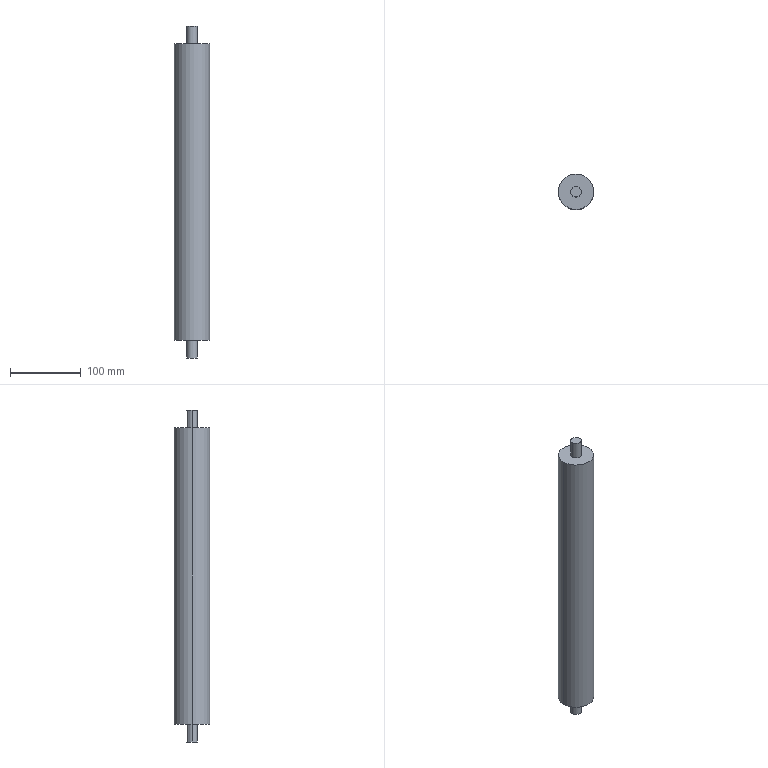Part | SolidWorks | features ICE 2, Extrusion 1 | 1 solid | 10 faces | box 50 x 50 x 470 mm | volume 833504 mm3 | cylinder 6 | plane 4 | commonest cylinder face diameters 15 x4 50 x2
STEP:
#1=CARTESIAN_POINT('',(-7.5,0.,-25.));
#2=VERTEX_POINT('',#1);
#3=CARTESIAN_POINT('',(7.5,0.,-25.));
#4=VERTEX_POINT('',#3);
#5=CARTESIAN_POINT('',(0.,0.,-25.));
#6=DIRECTION('',(0.,0.,-1.));
#7=DIRECTION('',(-1.,0.,0.));
#8=AXIS2_PLACEMENT_3D('',#5,#6,#7);
#9=CIRCLE('',#8,7.5);
#10=EDGE_CURVE('',#2,#4,#9,.T.);
#11=ORIENTED_EDGE('',*,*,#10,.F.);
#12=CARTESIAN_POINT('',(-7.5,0.,0.));
#13=VERTEX_POINT('',#12);
#14=CARTESIAN_POINT('',(-7.5,0.,-25.));
#15=DIRECTION('',(0.,0.,1.));
#16=VECTOR('',#15,1000.);
#17=LINE('',#14,#16);
#18=EDGE_CURVE('',#2,#13,#17,.T.);
#19=ORIENTED_EDGE('',*,*,#18,.T.);
#20=CARTESIAN_POINT('',(7.5,0.,0.));
#21=VERTEX_POINT('',#20);
#22=CARTESIAN_POINT('',(0.,0.,0.));
#23=DIRECTION('',(0.,0.,-1.));
#24=DIRECTION('',(-1.,0.,0.));
#25=AXIS2_PLACEMENT_3D('',#22,#23,#24);
#26=CIRCLE('',#25,7.5);
#27=EDGE_CURVE('',#13,#21,#26,.T.);
#28=ORIENTED_EDGE('',*,*,#27,.T.);
#29=CARTESIAN_POINT('',(7.5,0.,-25.));
#30=DIRECTION('',(0.,0.,1.));
#31=VECTOR('',#30,1000.);
#32=LINE('',#29,#31);
#33=EDGE_CURVE('',#4,#21,#32,.T.);
#34=ORIENTED_EDGE('',*,*,#33,.F.);
#35=EDGE_LOOP('',(#11,#19,#28,#34));
#36=FACE_OUTER_BOUND('',#35,.T.);
#37=CARTESIAN_POINT('',(0.,0.,-25.));
#38=DIRECTION('',(0.,0.,1.));
#39=DIRECTION('',(1.,0.,0.));
#40=AXIS2_PLACEMENT_3D('',#37,#38,#39);
#41=CYLINDRICAL_SURFACE('',#40,7.5);
#42=ADVANCED_FACE('',(#36),#41,.T.);
#43=CARTESIAN_POINT('',(7.5,0.,445.));
#44=VERTEX_POINT('',#43);
#45=CARTESIAN_POINT('',(-7.5,0.,445.));
#46=VERTEX_POINT('',#45);
#47=CARTESIAN_POINT('',(0.,0.,445.));
#48=DIRECTION('',(0.,0.,1.));
#49=DIRECTION('',(1.,0.,0.));
#50=AXIS2_PLACEMENT_3D('',#47,#48,#49);
#51=CIRCLE('',#50,7.5);
#52=EDGE_CURVE('',#44,#46,#51,.T.);
#53=ORIENTED_EDGE('',*,*,#52,.F.);
#54=CARTESIAN_POINT('',(7.5,0.,420.));
#55=VERTEX_POINT('',#54);
#56=CARTESIAN_POINT('',(7.5,0.,445.));
#57=DIRECTION('',(0.,0.,-1.));
#58=VECTOR('',#57,1000.);
#59=LINE('',#56,#58);
#60=EDGE_CURVE('',#44,#55,#59,.T.);
#61=ORIENTED_EDGE('',*,*,#60,.T.);
#62=CARTESIAN_POINT('',(-7.5,0.,420.));
#63=VERTEX_POINT('',#62);
#64=CARTESIAN_POINT('',(0.,0.,420.));
#65=DIRECTION('',(0.,0.,1.));
#66=DIRECTION('',(1.,0.,0.));
#67=AXIS2_PLACEMENT_3D('',#64,#65,#66);
#68=CIRCLE('',#67,7.5);
#69=EDGE_CURVE('',#55,#63,#68,.T.);
#70=ORIENTED_EDGE('',*,*,#69,.T.);
#71=CARTESIAN_POINT('',(-7.5,0.,445.));
#72=DIRECTION('',(0.,0.,-1.));
#73=VECTOR('',#72,1000.);
#74=LINE('',#71,#73);
#75=EDGE_CURVE('',#46,#63,#74,.T.);
#76=ORIENTED_EDGE('',*,*,#75,.F.);
#77=EDGE_LOOP('',(#53,#61,#70,#76));
#78=FACE_OUTER_BOUND('',#77,.T.);
#79=CARTESIAN_POINT('',(0.,0.,445.));
#80=DIRECTION('',(0.,0.,-1.));
#81=DIRECTION('',(-1.,0.,0.));
#82=AXIS2_PLACEMENT_3D('',#79,#80,#81);
#83=CYLINDRICAL_SURFACE('',#82,7.5);
#84=ADVANCED_FACE('',(#78),#83,.T.);
#85=CARTESIAN_POINT('',(25.,0.,420.));
#86=VERTEX_POINT('',#85);
#87=CARTESIAN_POINT('',(-25.,0.,420.));
#88=VERTEX_POINT('',#87);
#89=CARTESIAN_POINT('',(0.,0.,420.));
#90=DIRECTION('',(0.,0.,1.));
#91=DIRECTION('',(1.,0.,0.));
#92=AXIS2_PLACEMENT_3D('',#89,#90,#91);
#93=CIRCLE('',#92,25.);
#94=EDGE_CURVE('',#86,#88,#93,.T.);
#95=ORIENTED_EDGE('',*,*,#94,.F.);
#96=CARTESIAN_POINT('',(25.,0.,0.));
#97=VERTEX_POINT('',#96);
#98=CARTESIAN_POINT('',(25.,0.,420.));
#99=DIRECTION('',(0.,0.,-1.));
#100=VECTOR('',#99,1000.);
#101=LINE('',#98,#100);
#102=EDGE_CURVE('',#86,#97,#101,.T.);
#103=ORIENTED_EDGE('',*,*,#102,.T.);
#104=CARTESIAN_POINT('',(-25.,0.,0.));
#105=VERTEX_POINT('',#104);
#106=CARTESIAN_POINT('',(0.,0.,0.));
#107=DIRECTION('',(0.,0.,1.));
#108=DIRECTION('',(1.,0.,0.));
#109=AXIS2_PLACEMENT_3D('',#106,#107,#108);
#110=CIRCLE('',#109,25.);
#111=EDGE_CURVE('',#97,#105,#110,.T.);
#112=ORIENTED_EDGE('',*,*,#111,.T.);
#113=CARTESIAN_POINT('',(-25.,0.,420.));
#114=DIRECTION('',(0.,0.,-1.));
#115=VECTOR('',#114,1000.);
#116=LINE('',#113,#115);
#117=EDGE_CURVE('',#88,#105,#116,.T.);
#118=ORIENTED_EDGE('',*,*,#117,.F.);
#119=EDGE_LOOP('',(#95,#103,#112,#118));
#120=FACE_OUTER_BOUND('',#119,.T.);
#121=CARTESIAN_POINT('',(0.,0.,420.));
#122=DIRECTION('',(0.,0.,-1.));
#123=DIRECTION('',(-1.,0.,0.));
#124=AXIS2_PLACEMENT_3D('',#121,#122,#123);
#125=CYLINDRICAL_SURFACE('',#124,25.);
#126=ADVANCED_FACE('',(#120),#125,.T.);
#127=ORIENTED_EDGE('',*,*,#102,.F.);
#128=CARTESIAN_POINT('',(0.,0.,420.));
#129=DIRECTION('',(0.,0.,1.));
#130=DIRECTION('',(1.,0.,0.));
#131=AXIS2_PLACEMENT_3D('',#128,#129,#130);
#132=CIRCLE('',#131,25.);
#133=EDGE_CURVE('',#88,#86,#132,.T.);
#134=ORIENTED_EDGE('',*,*,#133,.F.);
#135=ORIENTED_EDGE('',*,*,#117,.T.);
#136=CARTESIAN_POINT('',(0.,0.,0.));
#137=DIRECTION('',(0.,0.,1.));
#138=DIRECTION('',(1.,0.,0.));
#139=AXIS2_PLACEMENT_3D('',#136,#137,#138);
#140=CIRCLE('',#139,25.);
#141=EDGE_CURVE('',#105,#97,#140,.T.);
#142=ORIENTED_EDGE('',*,*,#141,.T.);
#143=EDGE_LOOP('',(#127,#134,#135,#142));
#144=FACE_OUTER_BOUND('',#143,.T.);
#145=CARTESIAN_POINT('',(0.,0.,420.));
#146=DIRECTION('',(0.,0.,-1.));
#147=DIRECTION('',(-1.,0.,0.));
#148=AXIS2_PLACEMENT_3D('',#145,#146,#147);
#149=CYLINDRICAL_SURFACE('',#148,25.);
#150=ADVANCED_FACE('',(#144),#149,.T.);
#151=CARTESIAN_POINT('',(0.,0.,420.));
#152=DIRECTION('',(0.,0.,1.));
#153=DIRECTION('',(1.,0.,0.));
#154=AXIS2_PLACEMENT_3D('',#151,#152,#153);
#155=CIRCLE('',#154,7.5);
#156=EDGE_CURVE('',#63,#55,#155,.T.);
#157=ORIENTED_EDGE('',*,*,#156,.F.);
#158=ORIENTED_EDGE('',*,*,#69,.F.);
#159=EDGE_LOOP('',(#157,#158));
#160=FACE_BOUND('',#159,.T.);
#161=ORIENTED_EDGE('',*,*,#133,.T.);
#162=ORIENTED_EDGE('',*,*,#94,.T.);
#163=EDGE_LOOP('',(#161,#162));
#164=FACE_OUTER_BOUND('',#163,.T.);
#165=CARTESIAN_POINT('',(0.,0.,420.));
#166=DIRECTION('',(0.,0.,1.));
#167=DIRECTION('',(1.,0.,0.));
#168=AXIS2_PLACEMENT_3D('',#165,#166,#167);
#169=PLANE('',#168);
#170=ADVANCED_FACE('',(#160,#164),#169,.T.);
#171=CARTESIAN_POINT('',(0.,0.,0.));
#172=DIRECTION('',(0.,0.,-1.));
#173=DIRECTION('',(-1.,0.,0.));
#174=AXIS2_PLACEMENT_3D('',#171,#172,#173);
#175=CIRCLE('',#174,7.5);
#176=EDGE_CURVE('',#21,#13,#175,.T.);
#177=ORIENTED_EDGE('',*,*,#176,.F.);
#178=ORIENTED_EDGE('',*,*,#27,.F.);
#179=EDGE_LOOP('',(#177,#178));
#180=FACE_BOUND('',#179,.T.);
#181=ORIENTED_EDGE('',*,*,#141,.F.);
#182=ORIENTED_EDGE('',*,*,#111,.F.);
#183=EDGE_LOOP('',(#181,#182));
#184=FACE_OUTER_BOUND('',#183,.T.);
#185=CARTESIAN_POINT('',(0.,0.,0.));
#186=DIRECTION('',(0.,0.,1.));
#187=DIRECTION('',(1.,0.,0.));
#188=AXIS2_PLACEMENT_3D('',#185,#186,#187);
#189=PLANE('',#188);
#190=ADVANCED_FACE('',(#180,#184),#189,.F.);
#191=ORIENTED_EDGE('',*,*,#60,.F.);
#192=CARTESIAN_POINT('',(0.,0.,445.));
#193=DIRECTION('',(0.,0.,1.));
#194=DIRECTION('',(1.,0.,0.));
#195=AXIS2_PLACEMENT_3D('',#192,#193,#194);
#196=CIRCLE('',#195,7.5);
#197=EDGE_CURVE('',#46,#44,#196,.T.);
#198=ORIENTED_EDGE('',*,*,#197,.F.);
#199=ORIENTED_EDGE('',*,*,#75,.T.);
#200=ORIENTED_EDGE('',*,*,#156,.T.);
#201=EDGE_LOOP('',(#191,#198,#199,#200));
#202=FACE_OUTER_BOUND('',#201,.T.);
#203=CARTESIAN_POINT('',(0.,0.,445.));
#204=DIRECTION('',(0.,0.,-1.));
#205=DIRECTION('',(-1.,0.,0.));
#206=AXIS2_PLACEMENT_3D('',#203,#204,#205);
#207=CYLINDRICAL_SURFACE('',#206,7.5);
#208=ADVANCED_FACE('',(#202),#207,.T.);
#209=ORIENTED_EDGE('',*,*,#197,.T.);
#210=ORIENTED_EDGE('',*,*,#52,.T.);
#211=EDGE_LOOP('',(#209,#210));
#212=FACE_OUTER_BOUND('',#211,.T.);
#213=CARTESIAN_POINT('',(0.,0.,445.));
#214=DIRECTION('',(0.,0.,1.));
#215=DIRECTION('',(1.,0.,0.));
#216=AXIS2_PLACEMENT_3D('',#213,#214,#215);
#217=PLANE('',#216);
#218=ADVANCED_FACE('',(#212),#217,.T.);
#219=ORIENTED_EDGE('',*,*,#18,.F.);
#220=CARTESIAN_POINT('',(0.,0.,-25.));
#221=DIRECTION('',(0.,0.,-1.));
#222=DIRECTION('',(-1.,0.,0.));
#223=AXIS2_PLACEMENT_3D('',#220,#221,#222);
#224=CIRCLE('',#223,7.5);
#225=EDGE_CURVE('',#4,#2,#224,.T.);
#226=ORIENTED_EDGE('',*,*,#225,.F.);
#227=ORIENTED_EDGE('',*,*,#33,.T.);
#228=ORIENTED_EDGE('',*,*,#176,.T.);
#229=EDGE_LOOP('',(#219,#226,#227,#228));
#230=FACE_OUTER_BOUND('',#229,.T.);
#231=CARTESIAN_POINT('',(0.,0.,-25.));
#232=DIRECTION('',(0.,0.,1.));
#233=DIRECTION('',(1.,0.,0.));
#234=AXIS2_PLACEMENT_3D('',#231,#232,#233);
#235=CYLINDRICAL_SURFACE('',#234,7.5);
#236=ADVANCED_FACE('',(#230),#235,.T.);
#237=ORIENTED_EDGE('',*,*,#225,.T.);
#238=ORIENTED_EDGE('',*,*,#10,.T.);
#239=EDGE_LOOP('',(#237,#238));
#240=FACE_OUTER_BOUND('',#239,.T.);
#241=CARTESIAN_POINT('',(0.,0.,-25.));
#242=DIRECTION('',(0.,0.,-1.));
#243=DIRECTION('',(-1.,0.,0.));
#244=AXIS2_PLACEMENT_3D('',#241,#242,#243);
#245=PLANE('',#244);
#246=ADVANCED_FACE('',(#240),#245,.T.);
#247=CLOSED_SHELL('',(#42,#84,#126,#150,#170,#190,#208,#218,#236,#246));
#248=MANIFOLD_SOLID_BREP('',#247);
#249=CARTESIAN_POINT('',(0.,0.,0.));
#250=DIRECTION('',(0.,0.,1.));
#251=DIRECTION('',(1.,0.,0.));
#252=AXIS2_PLACEMENT_3D('',#249,#250,#251);
#253=(LENGTH_UNIT()NAMED_UNIT(*)SI_UNIT(.MILLI.,.METRE.));
#254=UNCERTAINTY_MEASURE_WITH_UNIT(LENGTH_MEASURE(0.00001),#253,'','');
#255=(NAMED_UNIT(*)PLANE_ANGLE_UNIT()SI_UNIT($,.RADIAN.));
#256=(NAMED_UNIT(*)SI_UNIT($,.STERADIAN.)SOLID_ANGLE_UNIT());
#257=(GEOMETRIC_REPRESENTATION_CONTEXT(3)GLOBAL_UNCERTAINTY_ASSIGNED_CONTEXT((#254))GLOBAL_UNIT_ASSIGNED_CONTEXT((#253,#255,#256))REPRESENTATION_CONTEXT('',''));
#258=ADVANCED_BREP_SHAPE_REPRESENTATION('',(#248,#252),#257);